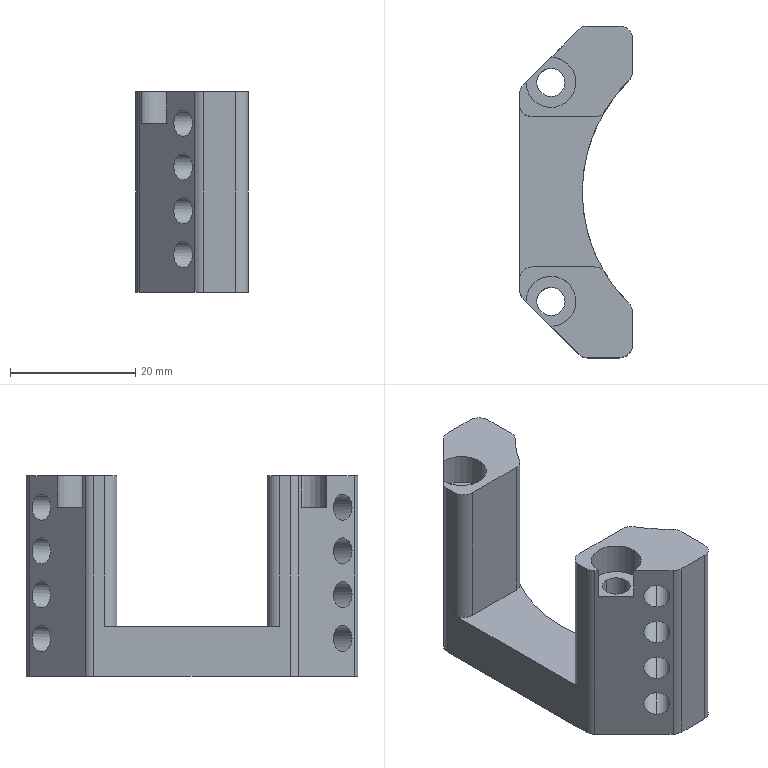Part | 1 solid | 50 faces | volume 11786 mm3 | cylinder 35 | plane 15 | commonest cylinder face diameters 4.2 x16 4 x12 4.5 x4 8 x2 50 x1